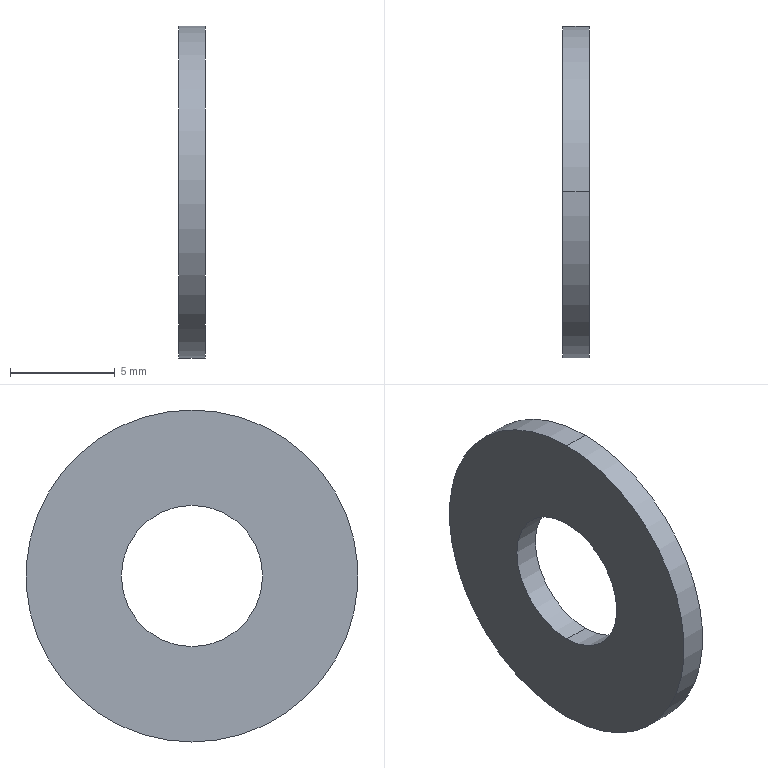Part | SolidWorks | features BaseBody 1 | 1 solid | 6 faces | box 1.245 x 15.875 x 15.875 mm | volume 201.725 mm3 | cylinder 4 | plane 2 | commonest cylinder face diameters 6.756 x2 15.875 x2
STEP:
#1=CARTESIAN_POINT('',(0.,0.,-7.938));
#2=VERTEX_POINT('',#1);
#3=CARTESIAN_POINT('',(0.,0.,7.938));
#4=VERTEX_POINT('',#3);
#5=CARTESIAN_POINT('',(0.,0.,0.));
#6=DIRECTION('',(1.,0.,0.));
#7=DIRECTION('',(0.,0.,1.));
#8=AXIS2_PLACEMENT_3D('',#5,#6,#7);
#9=CIRCLE('',#8,7.938);
#10=EDGE_CURVE('',#2,#4,#9,.T.);
#11=ORIENTED_EDGE('',*,*,#10,.F.);
#12=CARTESIAN_POINT('',(-1.245,0.,-7.938));
#13=VERTEX_POINT('',#12);
#14=CARTESIAN_POINT('',(0.,0.,-7.938));
#15=DIRECTION('',(-1.,0.,0.));
#16=VECTOR('',#15,1000.);
#17=LINE('',#14,#16);
#18=EDGE_CURVE('',#2,#13,#17,.T.);
#19=ORIENTED_EDGE('',*,*,#18,.T.);
#20=CARTESIAN_POINT('',(-1.245,0.,7.938));
#21=VERTEX_POINT('',#20);
#22=CARTESIAN_POINT('',(-1.245,0.,0.));
#23=DIRECTION('',(-1.,0.,0.));
#24=DIRECTION('',(0.,0.,1.));
#25=AXIS2_PLACEMENT_3D('',#22,#23,#24);
#26=CIRCLE('',#25,7.938);
#27=EDGE_CURVE('',#21,#13,#26,.T.);
#28=ORIENTED_EDGE('',*,*,#27,.F.);
#29=CARTESIAN_POINT('',(0.,0.,7.938));
#30=DIRECTION('',(-1.,0.,0.));
#31=VECTOR('',#30,1000.);
#32=LINE('',#29,#31);
#33=EDGE_CURVE('',#4,#21,#32,.T.);
#34=ORIENTED_EDGE('',*,*,#33,.F.);
#35=EDGE_LOOP('',(#11,#19,#28,#34));
#36=FACE_OUTER_BOUND('',#35,.T.);
#37=CARTESIAN_POINT('',(0.,0.,0.));
#38=DIRECTION('',(-1.,0.,0.));
#39=DIRECTION('',(0.,0.,1.));
#40=AXIS2_PLACEMENT_3D('',#37,#38,#39);
#41=CYLINDRICAL_SURFACE('',#40,7.938);
#42=ADVANCED_FACE('',(#36),#41,.T.);
#43=CARTESIAN_POINT('',(0.,0.,3.378));
#44=VERTEX_POINT('',#43);
#45=CARTESIAN_POINT('',(0.,0.,-3.378));
#46=VERTEX_POINT('',#45);
#47=CARTESIAN_POINT('',(0.,0.,0.));
#48=DIRECTION('',(1.,0.,0.));
#49=DIRECTION('',(0.,0.,1.));
#50=AXIS2_PLACEMENT_3D('',#47,#48,#49);
#51=CIRCLE('',#50,3.378);
#52=EDGE_CURVE('',#44,#46,#51,.T.);
#53=ORIENTED_EDGE('',*,*,#52,.T.);
#54=CARTESIAN_POINT('',(-1.245,0.,-3.378));
#55=VERTEX_POINT('',#54);
#56=CARTESIAN_POINT('',(0.,0.,-3.378));
#57=DIRECTION('',(-1.,0.,0.));
#58=VECTOR('',#57,1000.);
#59=LINE('',#56,#58);
#60=EDGE_CURVE('',#46,#55,#59,.T.);
#61=ORIENTED_EDGE('',*,*,#60,.T.);
#62=CARTESIAN_POINT('',(-1.245,0.,3.378));
#63=VERTEX_POINT('',#62);
#64=CARTESIAN_POINT('',(-1.245,0.,0.));
#65=DIRECTION('',(-1.,0.,0.));
#66=DIRECTION('',(0.,0.,1.));
#67=AXIS2_PLACEMENT_3D('',#64,#65,#66);
#68=CIRCLE('',#67,3.378);
#69=EDGE_CURVE('',#55,#63,#68,.T.);
#70=ORIENTED_EDGE('',*,*,#69,.T.);
#71=CARTESIAN_POINT('',(0.,0.,3.378));
#72=DIRECTION('',(-1.,0.,0.));
#73=VECTOR('',#72,1000.);
#74=LINE('',#71,#73);
#75=EDGE_CURVE('',#44,#63,#74,.T.);
#76=ORIENTED_EDGE('',*,*,#75,.F.);
#77=EDGE_LOOP('',(#53,#61,#70,#76));
#78=FACE_OUTER_BOUND('',#77,.T.);
#79=CARTESIAN_POINT('',(0.,0.,0.));
#80=DIRECTION('',(-1.,0.,0.));
#81=DIRECTION('',(0.,0.,1.));
#82=AXIS2_PLACEMENT_3D('',#79,#80,#81);
#83=CYLINDRICAL_SURFACE('',#82,3.378);
#84=ADVANCED_FACE('',(#78),#83,.F.);
#85=ORIENTED_EDGE('',*,*,#18,.F.);
#86=CARTESIAN_POINT('',(0.,0.,0.));
#87=DIRECTION('',(1.,0.,0.));
#88=DIRECTION('',(0.,0.,1.));
#89=AXIS2_PLACEMENT_3D('',#86,#87,#88);
#90=CIRCLE('',#89,7.938);
#91=EDGE_CURVE('',#4,#2,#90,.T.);
#92=ORIENTED_EDGE('',*,*,#91,.F.);
#93=ORIENTED_EDGE('',*,*,#33,.T.);
#94=CARTESIAN_POINT('',(-1.245,0.,0.));
#95=DIRECTION('',(-1.,0.,0.));
#96=DIRECTION('',(0.,0.,1.));
#97=AXIS2_PLACEMENT_3D('',#94,#95,#96);
#98=CIRCLE('',#97,7.938);
#99=EDGE_CURVE('',#13,#21,#98,.T.);
#100=ORIENTED_EDGE('',*,*,#99,.F.);
#101=EDGE_LOOP('',(#85,#92,#93,#100));
#102=FACE_OUTER_BOUND('',#101,.T.);
#103=CARTESIAN_POINT('',(0.,0.,0.));
#104=DIRECTION('',(-1.,0.,0.));
#105=DIRECTION('',(0.,0.,1.));
#106=AXIS2_PLACEMENT_3D('',#103,#104,#105);
#107=CYLINDRICAL_SURFACE('',#106,7.938);
#108=ADVANCED_FACE('',(#102),#107,.T.);
#109=ORIENTED_EDGE('',*,*,#52,.F.);
#110=CARTESIAN_POINT('',(0.,0.,0.));
#111=DIRECTION('',(1.,0.,0.));
#112=DIRECTION('',(0.,0.,1.));
#113=AXIS2_PLACEMENT_3D('',#110,#111,#112);
#114=CIRCLE('',#113,3.378);
#115=EDGE_CURVE('',#46,#44,#114,.T.);
#116=ORIENTED_EDGE('',*,*,#115,.F.);
#117=EDGE_LOOP('',(#109,#116));
#118=FACE_BOUND('',#117,.T.);
#119=ORIENTED_EDGE('',*,*,#91,.T.);
#120=ORIENTED_EDGE('',*,*,#10,.T.);
#121=EDGE_LOOP('',(#119,#120));
#122=FACE_OUTER_BOUND('',#121,.T.);
#123=CARTESIAN_POINT('',(0.,-8.033,-8.033));
#124=DIRECTION('',(-1.,0.,0.));
#125=DIRECTION('',(0.,0.,1.));
#126=AXIS2_PLACEMENT_3D('',#123,#124,#125);
#127=PLANE('',#126);
#128=ADVANCED_FACE('',(#118,#122),#127,.F.);
#129=CARTESIAN_POINT('',(-1.245,0.,0.));
#130=DIRECTION('',(-1.,0.,0.));
#131=DIRECTION('',(0.,0.,1.));
#132=AXIS2_PLACEMENT_3D('',#129,#130,#131);
#133=CIRCLE('',#132,3.378);
#134=EDGE_CURVE('',#63,#55,#133,.T.);
#135=ORIENTED_EDGE('',*,*,#134,.F.);
#136=ORIENTED_EDGE('',*,*,#69,.F.);
#137=EDGE_LOOP('',(#135,#136));
#138=FACE_BOUND('',#137,.T.);
#139=ORIENTED_EDGE('',*,*,#27,.T.);
#140=ORIENTED_EDGE('',*,*,#99,.T.);
#141=EDGE_LOOP('',(#139,#140));
#142=FACE_OUTER_BOUND('',#141,.T.);
#143=CARTESIAN_POINT('',(-1.245,-8.033,8.033));
#144=DIRECTION('',(1.,0.,0.));
#145=DIRECTION('',(0.,0.,-1.));
#146=AXIS2_PLACEMENT_3D('',#143,#144,#145);
#147=PLANE('',#146);
#148=ADVANCED_FACE('',(#138,#142),#147,.F.);
#149=ORIENTED_EDGE('',*,*,#60,.F.);
#150=ORIENTED_EDGE('',*,*,#115,.T.);
#151=ORIENTED_EDGE('',*,*,#75,.T.);
#152=ORIENTED_EDGE('',*,*,#134,.T.);
#153=EDGE_LOOP('',(#149,#150,#151,#152));
#154=FACE_OUTER_BOUND('',#153,.T.);
#155=CARTESIAN_POINT('',(0.,0.,0.));
#156=DIRECTION('',(-1.,0.,0.));
#157=DIRECTION('',(0.,0.,1.));
#158=AXIS2_PLACEMENT_3D('',#155,#156,#157);
#159=CYLINDRICAL_SURFACE('',#158,3.378);
#160=ADVANCED_FACE('',(#154),#159,.F.);
#161=CLOSED_SHELL('',(#42,#84,#108,#128,#148,#160));
#162=MANIFOLD_SOLID_BREP('',#161);
#163=CARTESIAN_POINT('',(0.,0.,0.));
#164=DIRECTION('',(0.,0.,1.));
#165=DIRECTION('',(1.,0.,0.));
#166=AXIS2_PLACEMENT_3D('',#163,#164,#165);
#167=(LENGTH_UNIT()NAMED_UNIT(*)SI_UNIT(.MILLI.,.METRE.));
#168=UNCERTAINTY_MEASURE_WITH_UNIT(LENGTH_MEASURE(0.00001),#167,'','');
#169=(NAMED_UNIT(*)PLANE_ANGLE_UNIT()SI_UNIT($,.RADIAN.));
#170=(NAMED_UNIT(*)SI_UNIT($,.STERADIAN.)SOLID_ANGLE_UNIT());
#171=(GEOMETRIC_REPRESENTATION_CONTEXT(3)GLOBAL_UNCERTAINTY_ASSIGNED_CONTEXT((#168))GLOBAL_UNIT_ASSIGNED_CONTEXT((#167,#169,#170))REPRESENTATION_CONTEXT('',''));
#172=ADVANCED_BREP_SHAPE_REPRESENTATION('',(#162,#166),#171);